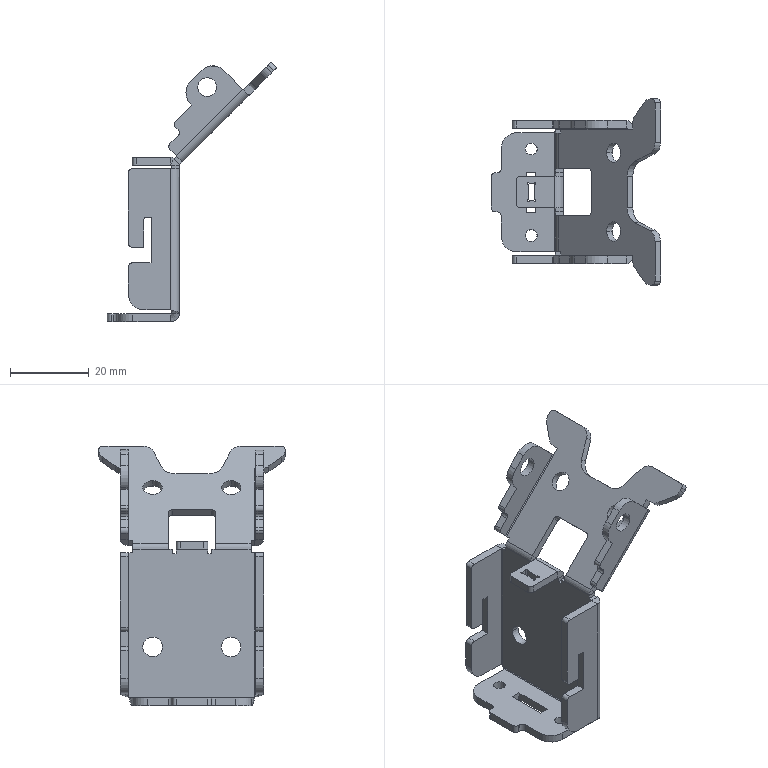Part | SolidWorks | features BaseBody 1 | 1 solid | 195 faces | box 43.104 x 47.401 x 66.159 mm | volume 7662 mm3 | plane 110 | cylinder 81 | spline 4 | commonest cylinder face diameters 2 x26 8 x11 0.4 x8 4.4 x8 5 x8 0.5 x6